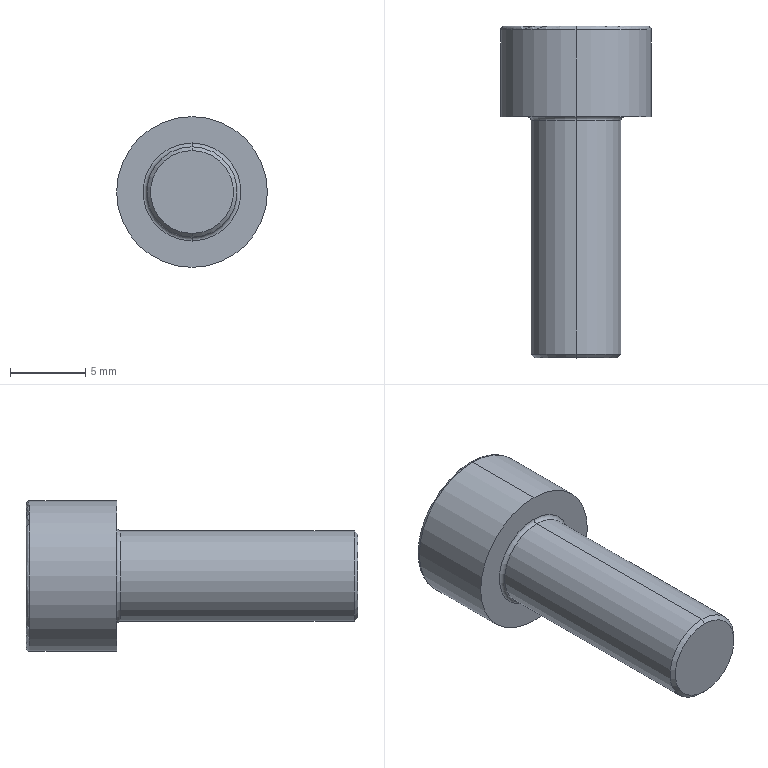Part | STEP file | 1 solid | 20 faces | box 10 x 22 x 10 mm | volume 857.945 mm3 | plane 10 | torus 4 | cylinder 4 | cone 2 | commonest cylinder face diameters 6 x2 10 x2
STEP:
#1=CARTESIAN_POINT('',(0.,-16.,-2.75));
#2=VERTEX_POINT('',#1);
#3=CARTESIAN_POINT('',(0.,-16.,2.75));
#4=VERTEX_POINT('',#3);
#5=CARTESIAN_POINT('',(0.,-16.,0.));
#6=DIRECTION('',(0.,-1.,0.));
#7=DIRECTION('',(0.,0.,-1.));
#8=AXIS2_PLACEMENT_3D('',#5,#6,#7);
#9=CIRCLE('',#8,2.75);
#10=EDGE_CURVE('',#2,#4,#9,.T.);
#11=ORIENTED_EDGE('',*,*,#10,.F.);
#12=CARTESIAN_POINT('',(0.,-15.75,-3.));
#13=VERTEX_POINT('',#12);
#14=CARTESIAN_POINT('',(0.,-16.,-2.75));
#15=DIRECTION('',(0.,0.7071,-0.7071));
#16=VECTOR('',#15,1000.);
#17=LINE('',#14,#16);
#18=EDGE_CURVE('',#2,#13,#17,.T.);
#19=ORIENTED_EDGE('',*,*,#18,.T.);
#20=CARTESIAN_POINT('',(0.,-15.75,3.));
#21=VERTEX_POINT('',#20);
#22=CARTESIAN_POINT('',(0.,-15.75,0.));
#23=DIRECTION('',(0.,1.,0.));
#24=DIRECTION('',(0.,0.,-1.));
#25=AXIS2_PLACEMENT_3D('',#22,#23,#24);
#26=CIRCLE('',#25,3.);
#27=EDGE_CURVE('',#21,#13,#26,.T.);
#28=ORIENTED_EDGE('',*,*,#27,.F.);
#29=CARTESIAN_POINT('',(0.,-16.,2.75));
#30=DIRECTION('',(0.,0.7071,0.7071));
#31=VECTOR('',#30,1000.);
#32=LINE('',#29,#31);
#33=EDGE_CURVE('',#4,#21,#32,.T.);
#34=ORIENTED_EDGE('',*,*,#33,.F.);
#35=EDGE_LOOP('',(#11,#19,#28,#34));
#36=FACE_OUTER_BOUND('',#35,.T.);
#37=CARTESIAN_POINT('',(0.,-16.,0.));
#38=DIRECTION('',(0.,1.,0.));
#39=DIRECTION('',(0.,0.,1.));
#40=AXIS2_PLACEMENT_3D('',#37,#38,#39);
#41=CONICAL_SURFACE('',#40,2.75,0.7854);
#42=ADVANCED_FACE('',(#36),#41,.T.);
#43=CARTESIAN_POINT('',(0.,5.75,-5.));
#44=VERTEX_POINT('',#43);
#45=CARTESIAN_POINT('',(0.,5.75,5.));
#46=VERTEX_POINT('',#45);
#47=CARTESIAN_POINT('',(0.,5.75,0.));
#48=DIRECTION('',(0.,-1.,0.));
#49=DIRECTION('',(0.,0.,1.));
#50=AXIS2_PLACEMENT_3D('',#47,#48,#49);
#51=CIRCLE('',#50,5.);
#52=EDGE_CURVE('',#44,#46,#51,.T.);
#53=ORIENTED_EDGE('',*,*,#52,.F.);
#54=CARTESIAN_POINT('',(0.,6.,-4.75));
#55=VERTEX_POINT('',#54);
#56=CARTESIAN_POINT('',(0.,5.75,-4.75));
#57=DIRECTION('',(1.,0.,0.));
#58=DIRECTION('',(0.,0.,-1.));
#59=AXIS2_PLACEMENT_3D('',#56,#57,#58);
#60=CIRCLE('',#59,0.25);
#61=EDGE_CURVE('',#44,#55,#60,.T.);
#62=ORIENTED_EDGE('',*,*,#61,.T.);
#63=CARTESIAN_POINT('',(0.,6.,4.75));
#64=VERTEX_POINT('',#63);
#65=CARTESIAN_POINT('',(0.,6.,0.));
#66=DIRECTION('',(0.,1.,0.));
#67=DIRECTION('',(0.,0.,1.));
#68=AXIS2_PLACEMENT_3D('',#65,#66,#67);
#69=CIRCLE('',#68,4.75);
#70=EDGE_CURVE('',#64,#55,#69,.T.);
#71=ORIENTED_EDGE('',*,*,#70,.F.);
#72=CARTESIAN_POINT('',(0.,5.75,4.75));
#73=DIRECTION('',(-1.,0.,0.));
#74=DIRECTION('',(0.,0.,1.));
#75=AXIS2_PLACEMENT_3D('',#72,#73,#74);
#76=CIRCLE('',#75,0.25);
#77=EDGE_CURVE('',#46,#64,#76,.T.);
#78=ORIENTED_EDGE('',*,*,#77,.F.);
#79=EDGE_LOOP('',(#53,#62,#71,#78));
#80=FACE_OUTER_BOUND('',#79,.T.);
#81=CARTESIAN_POINT('',(0.,5.75,0.));
#82=DIRECTION('',(0.,1.,0.));
#83=DIRECTION('',(0.,0.,1.));
#84=AXIS2_PLACEMENT_3D('',#81,#82,#83);
#85=TOROIDAL_SURFACE('',#84,4.75,0.25);
#86=ADVANCED_FACE('',(#80),#85,.T.);
#87=CARTESIAN_POINT('',(0.,-0.25,3.));
#88=VERTEX_POINT('',#87);
#89=CARTESIAN_POINT('',(0.,-0.25,-3.));
#90=VERTEX_POINT('',#89);
#91=CARTESIAN_POINT('',(0.,-0.25,0.));
#92=DIRECTION('',(0.,-1.,0.));
#93=DIRECTION('',(0.,0.,-1.));
#94=AXIS2_PLACEMENT_3D('',#91,#92,#93);
#95=CIRCLE('',#94,3.);
#96=EDGE_CURVE('',#88,#90,#95,.T.);
#97=ORIENTED_EDGE('',*,*,#96,.F.);
#98=CARTESIAN_POINT('',(0.,0.,3.25));
#99=VERTEX_POINT('',#98);
#100=CARTESIAN_POINT('',(0.,-0.25,3.25));
#101=DIRECTION('',(1.,0.,0.));
#102=DIRECTION('',(0.,0.,-1.));
#103=AXIS2_PLACEMENT_3D('',#100,#101,#102);
#104=CIRCLE('',#103,0.25);
#105=EDGE_CURVE('',#88,#99,#104,.T.);
#106=ORIENTED_EDGE('',*,*,#105,.T.);
#107=CARTESIAN_POINT('',(0.,0.,-3.25));
#108=VERTEX_POINT('',#107);
#109=CARTESIAN_POINT('',(0.,0.,0.));
#110=DIRECTION('',(0.,1.,0.));
#111=DIRECTION('',(0.,0.,-1.));
#112=AXIS2_PLACEMENT_3D('',#109,#110,#111);
#113=CIRCLE('',#112,3.25);
#114=EDGE_CURVE('',#108,#99,#113,.T.);
#115=ORIENTED_EDGE('',*,*,#114,.F.);
#116=CARTESIAN_POINT('',(0.,-0.25,-3.25));
#117=DIRECTION('',(-1.,0.,0.));
#118=DIRECTION('',(0.,0.,1.));
#119=AXIS2_PLACEMENT_3D('',#116,#117,#118);
#120=CIRCLE('',#119,0.25);
#121=EDGE_CURVE('',#90,#108,#120,.T.);
#122=ORIENTED_EDGE('',*,*,#121,.F.);
#123=EDGE_LOOP('',(#97,#106,#115,#122));
#124=FACE_OUTER_BOUND('',#123,.T.);
#125=CARTESIAN_POINT('',(0.,-0.25,0.));
#126=DIRECTION('',(0.,-1.,0.));
#127=DIRECTION('',(0.,0.,-1.));
#128=AXIS2_PLACEMENT_3D('',#125,#126,#127);
#129=TOROIDAL_SURFACE('',#128,3.25,0.25);
#130=ADVANCED_FACE('',(#124),#129,.F.);
#131=CARTESIAN_POINT('',(0.,-0.25,0.));
#132=DIRECTION('',(0.,-1.,0.));
#133=DIRECTION('',(0.,0.,-1.));
#134=AXIS2_PLACEMENT_3D('',#131,#132,#133);
#135=CIRCLE('',#134,3.);
#136=EDGE_CURVE('',#90,#88,#135,.T.);
#137=ORIENTED_EDGE('',*,*,#136,.T.);
#138=CARTESIAN_POINT('',(0.,0.,3.));
#139=DIRECTION('',(0.,-1.,0.));
#140=VECTOR('',#139,1000.);
#141=LINE('',#138,#140);
#142=EDGE_CURVE('',#88,#21,#141,.T.);
#143=ORIENTED_EDGE('',*,*,#142,.T.);
#144=ORIENTED_EDGE('',*,*,#27,.T.);
#145=CARTESIAN_POINT('',(0.,0.,-3.));
#146=DIRECTION('',(0.,-1.,0.));
#147=VECTOR('',#146,1000.);
#148=LINE('',#145,#147);
#149=EDGE_CURVE('',#90,#13,#148,.T.);
#150=ORIENTED_EDGE('',*,*,#149,.F.);
#151=EDGE_LOOP('',(#137,#143,#144,#150));
#152=FACE_OUTER_BOUND('',#151,.T.);
#153=CARTESIAN_POINT('',(0.,0.,0.));
#154=DIRECTION('',(0.,-1.,0.));
#155=DIRECTION('',(0.,0.,-1.));
#156=AXIS2_PLACEMENT_3D('',#153,#154,#155);
#157=CYLINDRICAL_SURFACE('',#156,3.);
#158=ADVANCED_FACE('',(#152),#157,.T.);
#159=ORIENTED_EDGE('',*,*,#52,.T.);
#160=CARTESIAN_POINT('',(0.,0.,5.));
#161=VERTEX_POINT('',#160);
#162=CARTESIAN_POINT('',(0.,0.,5.));
#163=DIRECTION('',(0.,-1.,0.));
#164=VECTOR('',#163,1000.);
#165=LINE('',#162,#164);
#166=EDGE_CURVE('',#46,#161,#165,.T.);
#167=ORIENTED_EDGE('',*,*,#166,.T.);
#168=CARTESIAN_POINT('',(0.,0.,-5.));
#169=VERTEX_POINT('',#168);
#170=CARTESIAN_POINT('',(0.,0.,0.));
#171=DIRECTION('',(0.,-1.,0.));
#172=DIRECTION('',(0.,0.,-1.));
#173=AXIS2_PLACEMENT_3D('',#170,#171,#172);
#174=CIRCLE('',#173,5.);
#175=EDGE_CURVE('',#169,#161,#174,.T.);
#176=ORIENTED_EDGE('',*,*,#175,.F.);
#177=CARTESIAN_POINT('',(0.,0.,-5.));
#178=DIRECTION('',(0.,-1.,0.));
#179=VECTOR('',#178,1000.);
#180=LINE('',#177,#179);
#181=EDGE_CURVE('',#44,#169,#180,.T.);
#182=ORIENTED_EDGE('',*,*,#181,.F.);
#183=EDGE_LOOP('',(#159,#167,#176,#182));
#184=FACE_OUTER_BOUND('',#183,.T.);
#185=CARTESIAN_POINT('',(0.,0.,0.));
#186=DIRECTION('',(0.,-1.,0.));
#187=DIRECTION('',(0.,0.,-1.));
#188=AXIS2_PLACEMENT_3D('',#185,#186,#187);
#189=CYLINDRICAL_SURFACE('',#188,5.);
#190=ADVANCED_FACE('',(#184),#189,.T.);
#191=ORIENTED_EDGE('',*,*,#70,.T.);
#192=CARTESIAN_POINT('',(0.,6.,0.));
#193=DIRECTION('',(0.,1.,0.));
#194=DIRECTION('',(0.,0.,1.));
#195=AXIS2_PLACEMENT_3D('',#192,#193,#194);
#196=CIRCLE('',#195,4.75);
#197=EDGE_CURVE('',#55,#64,#196,.T.);
#198=ORIENTED_EDGE('',*,*,#197,.T.);
#199=EDGE_LOOP('',(#191,#198));
#200=FACE_OUTER_BOUND('',#199,.T.);
#201=CARTESIAN_POINT('',(0.,6.,-2.887));
#202=VERTEX_POINT('',#201);
#203=CARTESIAN_POINT('',(-2.5,6.,-1.443));
#204=VERTEX_POINT('',#203);
#205=CARTESIAN_POINT('',(0.,6.,-2.887));
#206=DIRECTION('',(-0.866,0.,0.5));
#207=VECTOR('',#206,1000.);
#208=LINE('',#205,#207);
#209=EDGE_CURVE('',#202,#204,#208,.T.);
#210=ORIENTED_EDGE('',*,*,#209,.F.);
#211=CARTESIAN_POINT('',(2.5,6.,-1.443));
#212=VERTEX_POINT('',#211);
#213=CARTESIAN_POINT('',(2.5,6.,-1.443));
#214=DIRECTION('',(-0.866,0.,-0.5));
#215=VECTOR('',#214,1000.);
#216=LINE('',#213,#215);
#217=EDGE_CURVE('',#212,#202,#216,.T.);
#218=ORIENTED_EDGE('',*,*,#217,.F.);
#219=CARTESIAN_POINT('',(2.5,6.,1.443));
#220=VERTEX_POINT('',#219);
#221=CARTESIAN_POINT('',(2.5,6.,1.443));
#222=DIRECTION('',(0.,0.,-1.));
#223=VECTOR('',#222,1000.);
#224=LINE('',#221,#223);
#225=EDGE_CURVE('',#220,#212,#224,.T.);
#226=ORIENTED_EDGE('',*,*,#225,.F.);
#227=CARTESIAN_POINT('',(0.,6.,2.887));
#228=VERTEX_POINT('',#227);
#229=CARTESIAN_POINT('',(0.,6.,2.887));
#230=DIRECTION('',(0.866,0.,-0.5));
#231=VECTOR('',#230,1000.);
#232=LINE('',#229,#231);
#233=EDGE_CURVE('',#228,#220,#232,.T.);
#234=ORIENTED_EDGE('',*,*,#233,.F.);
#235=CARTESIAN_POINT('',(-2.5,6.,1.443));
#236=VERTEX_POINT('',#235);
#237=CARTESIAN_POINT('',(-2.5,6.,1.443));
#238=DIRECTION('',(0.866,0.,0.5));
#239=VECTOR('',#238,1000.);
#240=LINE('',#237,#239);
#241=EDGE_CURVE('',#236,#228,#240,.T.);
#242=ORIENTED_EDGE('',*,*,#241,.F.);
#243=CARTESIAN_POINT('',(-2.5,6.,-1.443));
#244=DIRECTION('',(0.,0.,1.));
#245=VECTOR('',#244,1000.);
#246=LINE('',#243,#245);
#247=EDGE_CURVE('',#204,#236,#246,.T.);
#248=ORIENTED_EDGE('',*,*,#247,.F.);
#249=EDGE_LOOP('',(#210,#218,#226,#234,#242,#248));
#250=FACE_BOUND('',#249,.T.);
#251=CARTESIAN_POINT('',(0.,6.,0.));
#252=DIRECTION('',(0.,1.,0.));
#253=DIRECTION('',(0.,0.,1.));
#254=AXIS2_PLACEMENT_3D('',#251,#252,#253);
#255=PLANE('',#254);
#256=ADVANCED_FACE('',(#200,#250),#255,.T.);
#257=ORIENTED_EDGE('',*,*,#166,.F.);
#258=CARTESIAN_POINT('',(0.,5.75,0.));
#259=DIRECTION('',(0.,-1.,0.));
#260=DIRECTION('',(0.,0.,1.));
#261=AXIS2_PLACEMENT_3D('',#258,#259,#260);
#262=CIRCLE('',#261,5.);
#263=EDGE_CURVE('',#46,#44,#262,.T.);
#264=ORIENTED_EDGE('',*,*,#263,.T.);
#265=ORIENTED_EDGE('',*,*,#181,.T.);
#266=CARTESIAN_POINT('',(0.,0.,0.));
#267=DIRECTION('',(0.,-1.,0.));
#268=DIRECTION('',(0.,0.,-1.));
#269=AXIS2_PLACEMENT_3D('',#266,#267,#268);
#270=CIRCLE('',#269,5.);
#271=EDGE_CURVE('',#161,#169,#270,.T.);
#272=ORIENTED_EDGE('',*,*,#271,.F.);
#273=EDGE_LOOP('',(#257,#264,#265,#272));
#274=FACE_OUTER_BOUND('',#273,.T.);
#275=CARTESIAN_POINT('',(0.,0.,0.));
#276=DIRECTION('',(0.,-1.,0.));
#277=DIRECTION('',(0.,0.,-1.));
#278=AXIS2_PLACEMENT_3D('',#275,#276,#277);
#279=CYLINDRICAL_SURFACE('',#278,5.);
#280=ADVANCED_FACE('',(#274),#279,.T.);
#281=ORIENTED_EDGE('',*,*,#114,.T.);
#282=CARTESIAN_POINT('',(0.,0.,0.));
#283=DIRECTION('',(0.,1.,0.));
#284=DIRECTION('',(0.,0.,-1.));
#285=AXIS2_PLACEMENT_3D('',#282,#283,#284);
#286=CIRCLE('',#285,3.25);
#287=EDGE_CURVE('',#99,#108,#286,.T.);
#288=ORIENTED_EDGE('',*,*,#287,.T.);
#289=EDGE_LOOP('',(#281,#288));
#290=FACE_BOUND('',#289,.T.);
#291=ORIENTED_EDGE('',*,*,#175,.T.);
#292=ORIENTED_EDGE('',*,*,#271,.T.);
#293=EDGE_LOOP('',(#291,#292));
#294=FACE_OUTER_BOUND('',#293,.T.);
#295=CARTESIAN_POINT('',(5.,0.,0.));
#296=DIRECTION('',(0.,-1.,0.));
#297=DIRECTION('',(0.,0.,-1.));
#298=AXIS2_PLACEMENT_3D('',#295,#296,#297);
#299=PLANE('',#298);
#300=ADVANCED_FACE('',(#290,#294),#299,.T.);
#301=ORIENTED_EDGE('',*,*,#142,.F.);
#302=ORIENTED_EDGE('',*,*,#96,.T.);
#303=ORIENTED_EDGE('',*,*,#149,.T.);
#304=CARTESIAN_POINT('',(0.,-15.75,0.));
#305=DIRECTION('',(0.,1.,0.));
#306=DIRECTION('',(0.,0.,-1.));
#307=AXIS2_PLACEMENT_3D('',#304,#305,#306);
#308=CIRCLE('',#307,3.);
#309=EDGE_CURVE('',#13,#21,#308,.T.);
#310=ORIENTED_EDGE('',*,*,#309,.T.);
#311=EDGE_LOOP('',(#301,#302,#303,#310));
#312=FACE_OUTER_BOUND('',#311,.T.);
#313=CARTESIAN_POINT('',(0.,0.,0.));
#314=DIRECTION('',(0.,-1.,0.));
#315=DIRECTION('',(0.,0.,-1.));
#316=AXIS2_PLACEMENT_3D('',#313,#314,#315);
#317=CYLINDRICAL_SURFACE('',#316,3.);
#318=ADVANCED_FACE('',(#312),#317,.T.);
#319=CARTESIAN_POINT('',(0.,-16.,0.));
#320=DIRECTION('',(0.,-1.,0.));
#321=DIRECTION('',(0.,0.,-1.));
#322=AXIS2_PLACEMENT_3D('',#319,#320,#321);
#323=CIRCLE('',#322,2.75);
#324=EDGE_CURVE('',#4,#2,#323,.T.);
#325=ORIENTED_EDGE('',*,*,#324,.T.);
#326=ORIENTED_EDGE('',*,*,#10,.T.);
#327=EDGE_LOOP('',(#325,#326));
#328=FACE_OUTER_BOUND('',#327,.T.);
#329=CARTESIAN_POINT('',(3.,-16.,0.));
#330=DIRECTION('',(0.,-1.,0.));
#331=DIRECTION('',(0.,0.,-1.));
#332=AXIS2_PLACEMENT_3D('',#329,#330,#331);
#333=PLANE('',#332);
#334=ADVANCED_FACE('',(#328),#333,.T.);
#335=ORIENTED_EDGE('',*,*,#209,.T.);
#336=CARTESIAN_POINT('',(-2.5,3.,-1.443));
#337=VERTEX_POINT('',#336);
#338=CARTESIAN_POINT('',(-2.5,3.,-1.443));
#339=DIRECTION('',(0.,1.,0.));
#340=VECTOR('',#339,1000.);
#341=LINE('',#338,#340);
#342=EDGE_CURVE('',#337,#204,#341,.T.);
#343=ORIENTED_EDGE('',*,*,#342,.F.);
#344=CARTESIAN_POINT('',(0.,3.,-2.887));
#345=VERTEX_POINT('',#344);
#346=CARTESIAN_POINT('',(0.,3.,-2.887));
#347=DIRECTION('',(-0.866,0.,0.5));
#348=VECTOR('',#347,1000.);
#349=LINE('',#346,#348);
#350=EDGE_CURVE('',#345,#337,#349,.T.);
#351=ORIENTED_EDGE('',*,*,#350,.F.);
#352=CARTESIAN_POINT('',(0.,3.,-2.887));
#353=DIRECTION('',(0.,1.,0.));
#354=VECTOR('',#353,1000.);
#355=LINE('',#352,#354);
#356=EDGE_CURVE('',#345,#202,#355,.T.);
#357=ORIENTED_EDGE('',*,*,#356,.T.);
#358=EDGE_LOOP('',(#335,#343,#351,#357));
#359=FACE_OUTER_BOUND('',#358,.T.);
#360=CARTESIAN_POINT('',(0.,3.,-2.887));
#361=DIRECTION('',(-0.5,0.,-0.866));
#362=DIRECTION('',(-0.866,0.,0.5));
#363=AXIS2_PLACEMENT_3D('',#360,#361,#362);
#364=PLANE('',#363);
#365=ADVANCED_FACE('',(#359),#364,.F.);
#366=ORIENTED_EDGE('',*,*,#217,.T.);
#367=ORIENTED_EDGE('',*,*,#356,.F.);
#368=CARTESIAN_POINT('',(2.5,3.,-1.443));
#369=VERTEX_POINT('',#368);
#370=CARTESIAN_POINT('',(2.5,3.,-1.443));
#371=DIRECTION('',(-0.866,0.,-0.5));
#372=VECTOR('',#371,1000.);
#373=LINE('',#370,#372);
#374=EDGE_CURVE('',#369,#345,#373,.T.);
#375=ORIENTED_EDGE('',*,*,#374,.F.);
#376=CARTESIAN_POINT('',(2.5,3.,-1.443));
#377=DIRECTION('',(0.,1.,0.));
#378=VECTOR('',#377,1000.);
#379=LINE('',#376,#378);
#380=EDGE_CURVE('',#369,#212,#379,.T.);
#381=ORIENTED_EDGE('',*,*,#380,.T.);
#382=EDGE_LOOP('',(#366,#367,#375,#381));
#383=FACE_OUTER_BOUND('',#382,.T.);
#384=CARTESIAN_POINT('',(2.5,3.,-1.443));
#385=DIRECTION('',(0.5,0.,-0.866));
#386=DIRECTION('',(-0.866,0.,-0.5));
#387=AXIS2_PLACEMENT_3D('',#384,#385,#386);
#388=PLANE('',#387);
#389=ADVANCED_FACE('',(#383),#388,.F.);
#390=ORIENTED_EDGE('',*,*,#225,.T.);
#391=ORIENTED_EDGE('',*,*,#380,.F.);
#392=CARTESIAN_POINT('',(2.5,3.,1.443));
#393=VERTEX_POINT('',#392);
#394=CARTESIAN_POINT('',(2.5,3.,1.443));
#395=DIRECTION('',(0.,0.,-1.));
#396=VECTOR('',#395,1000.);
#397=LINE('',#394,#396);
#398=EDGE_CURVE('',#393,#369,#397,.T.);
#399=ORIENTED_EDGE('',*,*,#398,.F.);
#400=CARTESIAN_POINT('',(2.5,3.,1.443));
#401=DIRECTION('',(0.,1.,0.));
#402=VECTOR('',#401,1000.);
#403=LINE('',#400,#402);
#404=EDGE_CURVE('',#393,#220,#403,.T.);
#405=ORIENTED_EDGE('',*,*,#404,.T.);
#406=EDGE_LOOP('',(#390,#391,#399,#405));
#407=FACE_OUTER_BOUND('',#406,.T.);
#408=CARTESIAN_POINT('',(2.5,3.,1.443));
#409=DIRECTION('',(1.,0.,0.));
#410=DIRECTION('',(0.,0.,-1.));
#411=AXIS2_PLACEMENT_3D('',#408,#409,#410);
#412=PLANE('',#411);
#413=ADVANCED_FACE('',(#407),#412,.F.);
#414=ORIENTED_EDGE('',*,*,#233,.T.);
#415=ORIENTED_EDGE('',*,*,#404,.F.);
#416=CARTESIAN_POINT('',(0.,3.,2.887));
#417=VERTEX_POINT('',#416);
#418=CARTESIAN_POINT('',(0.,3.,2.887));
#419=DIRECTION('',(0.866,0.,-0.5));
#420=VECTOR('',#419,1000.);
#421=LINE('',#418,#420);
#422=EDGE_CURVE('',#417,#393,#421,.T.);
#423=ORIENTED_EDGE('',*,*,#422,.F.);
#424=CARTESIAN_POINT('',(0.,3.,2.887));
#425=DIRECTION('',(0.,1.,0.));
#426=VECTOR('',#425,1000.);
#427=LINE('',#424,#426);
#428=EDGE_CURVE('',#417,#228,#427,.T.);
#429=ORIENTED_EDGE('',*,*,#428,.T.);
#430=EDGE_LOOP('',(#414,#415,#423,#429));
#431=FACE_OUTER_BOUND('',#430,.T.);
#432=CARTESIAN_POINT('',(0.,3.,2.887));
#433=DIRECTION('',(0.5,0.,0.866));
#434=DIRECTION('',(0.866,0.,-0.5));
#435=AXIS2_PLACEMENT_3D('',#432,#433,#434);
#436=PLANE('',#435);
#437=ADVANCED_FACE('',(#431),#436,.F.);
#438=ORIENTED_EDGE('',*,*,#241,.T.);
#439=ORIENTED_EDGE('',*,*,#428,.F.);
#440=CARTESIAN_POINT('',(-2.5,3.,1.443));
#441=VERTEX_POINT('',#440);
#442=CARTESIAN_POINT('',(-2.5,3.,1.443));
#443=DIRECTION('',(0.866,0.,0.5));
#444=VECTOR('',#443,1000.);
#445=LINE('',#442,#444);
#446=EDGE_CURVE('',#441,#417,#445,.T.);
#447=ORIENTED_EDGE('',*,*,#446,.F.);
#448=CARTESIAN_POINT('',(-2.5,3.,1.443));
#449=DIRECTION('',(0.,1.,0.));
#450=VECTOR('',#449,1000.);
#451=LINE('',#448,#450);
#452=EDGE_CURVE('',#441,#236,#451,.T.);
#453=ORIENTED_EDGE('',*,*,#452,.T.);
#454=EDGE_LOOP('',(#438,#439,#447,#453));
#455=FACE_OUTER_BOUND('',#454,.T.);
#456=CARTESIAN_POINT('',(-2.5,3.,1.443));
#457=DIRECTION('',(-0.5,0.,0.866));
#458=DIRECTION('',(0.866,0.,0.5));
#459=AXIS2_PLACEMENT_3D('',#456,#457,#458);
#460=PLANE('',#459);
#461=ADVANCED_FACE('',(#455),#460,.F.);
#462=ORIENTED_EDGE('',*,*,#247,.T.);
#463=ORIENTED_EDGE('',*,*,#452,.F.);
#464=CARTESIAN_POINT('',(-2.5,3.,-1.443));
#465=DIRECTION('',(0.,0.,1.));
#466=VECTOR('',#465,1000.);
#467=LINE('',#464,#466);
#468=EDGE_CURVE('',#337,#441,#467,.T.);
#469=ORIENTED_EDGE('',*,*,#468,.F.);
#470=ORIENTED_EDGE('',*,*,#342,.T.);
#471=EDGE_LOOP('',(#462,#463,#469,#470));
#472=FACE_OUTER_BOUND('',#471,.T.);
#473=CARTESIAN_POINT('',(-2.5,3.,-1.443));
#474=DIRECTION('',(-1.,0.,0.));
#475=DIRECTION('',(0.,0.,1.));
#476=AXIS2_PLACEMENT_3D('',#473,#474,#475);
#477=PLANE('',#476);
#478=ADVANCED_FACE('',(#472),#477,.F.);
#479=ORIENTED_EDGE('',*,*,#350,.T.);
#480=ORIENTED_EDGE('',*,*,#468,.T.);
#481=ORIENTED_EDGE('',*,*,#446,.T.);
#482=ORIENTED_EDGE('',*,*,#422,.T.);
#483=ORIENTED_EDGE('',*,*,#398,.T.);
#484=ORIENTED_EDGE('',*,*,#374,.T.);
#485=EDGE_LOOP('',(#479,#480,#481,#482,#483,#484));
#486=FACE_OUTER_BOUND('',#485,.T.);
#487=CARTESIAN_POINT('',(0.,3.,0.));
#488=DIRECTION('',(0.,1.,0.));
#489=DIRECTION('',(0.,0.,1.));
#490=AXIS2_PLACEMENT_3D('',#487,#488,#489);
#491=PLANE('',#490);
#492=ADVANCED_FACE('',(#486),#491,.T.);
#493=ORIENTED_EDGE('',*,*,#105,.F.);
#494=ORIENTED_EDGE('',*,*,#136,.F.);
#495=ORIENTED_EDGE('',*,*,#121,.T.);
#496=ORIENTED_EDGE('',*,*,#287,.F.);
#497=EDGE_LOOP('',(#493,#494,#495,#496));
#498=FACE_OUTER_BOUND('',#497,.T.);
#499=CARTESIAN_POINT('',(0.,-0.25,0.));
#500=DIRECTION('',(0.,-1.,0.));
#501=DIRECTION('',(0.,0.,-1.));
#502=AXIS2_PLACEMENT_3D('',#499,#500,#501);
#503=TOROIDAL_SURFACE('',#502,3.25,0.25);
#504=ADVANCED_FACE('',(#498),#503,.F.);
#505=ORIENTED_EDGE('',*,*,#61,.F.);
#506=ORIENTED_EDGE('',*,*,#263,.F.);
#507=ORIENTED_EDGE('',*,*,#77,.T.);
#508=ORIENTED_EDGE('',*,*,#197,.F.);
#509=EDGE_LOOP('',(#505,#506,#507,#508));
#510=FACE_OUTER_BOUND('',#509,.T.);
#511=CARTESIAN_POINT('',(0.,5.75,0.));
#512=DIRECTION('',(0.,1.,0.));
#513=DIRECTION('',(0.,0.,1.));
#514=AXIS2_PLACEMENT_3D('',#511,#512,#513);
#515=TOROIDAL_SURFACE('',#514,4.75,0.25);
#516=ADVANCED_FACE('',(#510),#515,.T.);
#517=ORIENTED_EDGE('',*,*,#18,.F.);
#518=ORIENTED_EDGE('',*,*,#324,.F.);
#519=ORIENTED_EDGE('',*,*,#33,.T.);
#520=ORIENTED_EDGE('',*,*,#309,.F.);
#521=EDGE_LOOP('',(#517,#518,#519,#520));
#522=FACE_OUTER_BOUND('',#521,.T.);
#523=CARTESIAN_POINT('',(0.,-16.,0.));
#524=DIRECTION('',(0.,1.,0.));
#525=DIRECTION('',(0.,0.,1.));
#526=AXIS2_PLACEMENT_3D('',#523,#524,#525);
#527=CONICAL_SURFACE('',#526,2.75,0.7854);
#528=ADVANCED_FACE('',(#522),#527,.T.);
#529=CLOSED_SHELL('',(#42,#86,#130,#158,#190,#256,#280,#300,#318,#334,#365,#389,#413,#437,#461,#478,#492,#504,#516,#528));
#530=MANIFOLD_SOLID_BREP('',#529);
#531=CARTESIAN_POINT('',(0.,0.,0.));
#532=DIRECTION('',(0.,0.,1.));
#533=DIRECTION('',(1.,0.,0.));
#534=AXIS2_PLACEMENT_3D('',#531,#532,#533);
#535=(LENGTH_UNIT()NAMED_UNIT(*)SI_UNIT(.MILLI.,.METRE.));
#536=UNCERTAINTY_MEASURE_WITH_UNIT(LENGTH_MEASURE(0.00001),#535,'','');
#537=(NAMED_UNIT(*)PLANE_ANGLE_UNIT()SI_UNIT($,.RADIAN.));
#538=(NAMED_UNIT(*)SI_UNIT($,.STERADIAN.)SOLID_ANGLE_UNIT());
#539=(GEOMETRIC_REPRESENTATION_CONTEXT(3)GLOBAL_UNCERTAINTY_ASSIGNED_CONTEXT((#536))GLOBAL_UNIT_ASSIGNED_CONTEXT((#535,#537,#538))REPRESENTATION_CONTEXT('',''));
#540=ADVANCED_BREP_SHAPE_REPRESENTATION('',(#530,#534),#539);